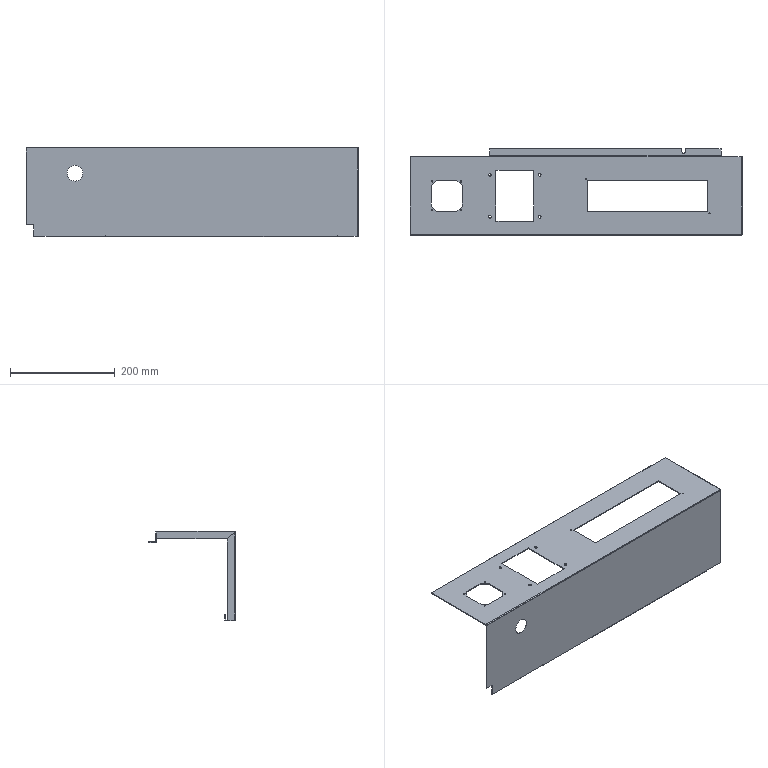Part | STEP file | FHD-021-001-D rack welded part D | 1 solid | 91 faces | box 633.5 x 165 x 171.5 mm | volume 312915 mm3 | plane 63 | cylinder 26 | spline 2 | commonest cylinder face diameters 0.4 x7 3.4 x7 2.5 x4 5 x4 2 x2 6 x1